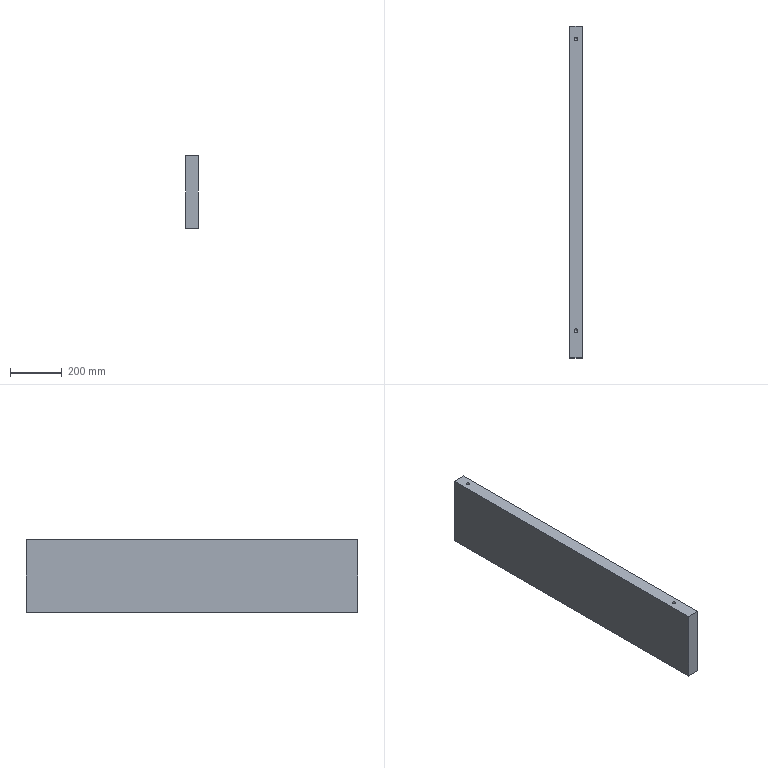Part | NX | features 29 2 | 1 solid | 16 faces | box 50 x 1280 x 280.5 mm | volume 17921318 mm3 | plane 6 | cylinder 5 | cone 5 | commonest cylinder face diameters 14.1 x5
STEP:
#1=CARTESIAN_POINT('',(2407.05,622.5,-493.5));
#2=VERTEX_POINT('',#1);
#3=CARTESIAN_POINT('',(2400.,622.5,-493.5));
#4=DIRECTION('',(0.,0.,1.));
#5=DIRECTION('',(1.,0.,0.));
#6=AXIS2_PLACEMENT_3D('',#3,#4,#5);
#7=CIRCLE('',#6,7.05);
#8=EDGE_CURVE('',#2,#2,#7,.T.);
#9=ORIENTED_EDGE('',*,*,#8,.T.);
#10=EDGE_LOOP('',(#9));
#11=FACE_BOUND('',#10,.T.);
#12=CARTESIAN_POINT('',(2375.,-607.5,-493.5));
#13=VERTEX_POINT('',#12);
#14=CARTESIAN_POINT('',(2425.,-607.5,-493.5));
#15=VERTEX_POINT('',#14);
#16=CARTESIAN_POINT('',(2330.,-607.5,-493.5));
#17=DIRECTION('',(1.,0.,0.));
#18=VECTOR('',#17,1000.);
#19=LINE('',#16,#18);
#20=EDGE_CURVE('',#13,#15,#19,.T.);
#21=ORIENTED_EDGE('',*,*,#20,.F.);
#22=CARTESIAN_POINT('',(2375.,672.5,-493.5));
#23=VERTEX_POINT('',#22);
#24=CARTESIAN_POINT('',(2375.,193.,-493.5));
#25=DIRECTION('',(0.,-1.,0.));
#26=VECTOR('',#25,1000.);
#27=LINE('',#24,#26);
#28=EDGE_CURVE('',#23,#13,#27,.T.);
#29=ORIENTED_EDGE('',*,*,#28,.F.);
#30=CARTESIAN_POINT('',(2425.,672.5,-493.5));
#31=VERTEX_POINT('',#30);
#32=CARTESIAN_POINT('',(1932.5,672.5,-493.5));
#33=DIRECTION('',(1.,0.,0.));
#34=VECTOR('',#33,1000.);
#35=LINE('',#32,#34);
#36=EDGE_CURVE('',#23,#31,#35,.T.);
#37=ORIENTED_EDGE('',*,*,#36,.T.);
#38=CARTESIAN_POINT('',(2425.,193.,-493.5));
#39=DIRECTION('',(0.,1.,0.));
#40=VECTOR('',#39,1000.);
#41=LINE('',#38,#40);
#42=EDGE_CURVE('',#15,#31,#41,.T.);
#43=ORIENTED_EDGE('',*,*,#42,.F.);
#44=EDGE_LOOP('',(#21,#29,#37,#43));
#45=FACE_BOUND('',#44,.T.);
#46=CARTESIAN_POINT('',(2407.05,-502.5,-493.5));
#47=VERTEX_POINT('',#46);
#48=CARTESIAN_POINT('',(2400.,-502.5,-493.5));
#49=DIRECTION('',(0.,0.,1.));
#50=DIRECTION('',(1.,0.,0.));
#51=AXIS2_PLACEMENT_3D('',#48,#49,#50);
#52=CIRCLE('',#51,7.05);
#53=EDGE_CURVE('',#47,#47,#52,.T.);
#54=ORIENTED_EDGE('',*,*,#53,.T.);
#55=EDGE_LOOP('',(#54));
#56=FACE_BOUND('',#55,.T.);
#57=CARTESIAN_POINT('',(2407.05,32.5,-493.5));
#58=VERTEX_POINT('',#57);
#59=CARTESIAN_POINT('',(2400.,32.5,-493.5));
#60=DIRECTION('',(0.,0.,1.));
#61=DIRECTION('',(1.,0.,0.));
#62=AXIS2_PLACEMENT_3D('',#59,#60,#61);
#63=CIRCLE('',#62,7.05);
#64=EDGE_CURVE('',#58,#58,#63,.T.);
#65=ORIENTED_EDGE('',*,*,#64,.T.);
#66=EDGE_LOOP('',(#65));
#67=FACE_BOUND('',#66,.T.);
#68=CARTESIAN_POINT('',(1945.,0.,-493.5));
#69=DIRECTION('',(0.,0.,-1.));
#70=DIRECTION('',(1.,0.,0.));
#71=AXIS2_PLACEMENT_3D('',#68,#69,#70);
#72=PLANE('',#71);
#73=ADVANCED_FACE('',(#11,#45,#56,#67),#72,.T.);
#74=CARTESIAN_POINT('',(2407.05,622.5,-213.));
#75=VERTEX_POINT('',#74);
#76=CARTESIAN_POINT('',(2400.,622.5,-213.));
#77=DIRECTION('',(0.,0.,-1.));
#78=DIRECTION('',(1.,0.,0.));
#79=AXIS2_PLACEMENT_3D('',#76,#77,#78);
#80=CIRCLE('',#79,7.05);
#81=EDGE_CURVE('',#75,#75,#80,.T.);
#82=ORIENTED_EDGE('',*,*,#81,.T.);
#83=EDGE_LOOP('',(#82));
#84=FACE_BOUND('',#83,.T.);
#85=CARTESIAN_POINT('',(2425.,-607.5,-213.));
#86=VERTEX_POINT('',#85);
#87=CARTESIAN_POINT('',(2375.,-607.5,-213.));
#88=VERTEX_POINT('',#87);
#89=CARTESIAN_POINT('',(2330.,-607.5,-213.));
#90=DIRECTION('',(-1.,0.,0.));
#91=VECTOR('',#90,1000.);
#92=LINE('',#89,#91);
#93=EDGE_CURVE('',#86,#88,#92,.T.);
#94=ORIENTED_EDGE('',*,*,#93,.F.);
#95=CARTESIAN_POINT('',(2425.,672.5,-213.));
#96=VERTEX_POINT('',#95);
#97=CARTESIAN_POINT('',(2425.,193.,-213.));
#98=DIRECTION('',(0.,-1.,0.));
#99=VECTOR('',#98,1000.);
#100=LINE('',#97,#99);
#101=EDGE_CURVE('',#96,#86,#100,.T.);
#102=ORIENTED_EDGE('',*,*,#101,.F.);
#103=CARTESIAN_POINT('',(2375.,672.5,-213.));
#104=VERTEX_POINT('',#103);
#105=CARTESIAN_POINT('',(1932.5,672.5,-213.));
#106=DIRECTION('',(-1.,0.,0.));
#107=VECTOR('',#106,1000.);
#108=LINE('',#105,#107);
#109=EDGE_CURVE('',#96,#104,#108,.T.);
#110=ORIENTED_EDGE('',*,*,#109,.T.);
#111=CARTESIAN_POINT('',(2375.,193.,-213.));
#112=DIRECTION('',(0.,1.,0.));
#113=VECTOR('',#112,1000.);
#114=LINE('',#111,#113);
#115=EDGE_CURVE('',#88,#104,#114,.T.);
#116=ORIENTED_EDGE('',*,*,#115,.F.);
#117=EDGE_LOOP('',(#94,#102,#110,#116));
#118=FACE_BOUND('',#117,.T.);
#119=CARTESIAN_POINT('',(2407.05,-502.5,-213.));
#120=VERTEX_POINT('',#119);
#121=CARTESIAN_POINT('',(2400.,-502.5,-213.));
#122=DIRECTION('',(0.,0.,-1.));
#123=DIRECTION('',(1.,0.,0.));
#124=AXIS2_PLACEMENT_3D('',#121,#122,#123);
#125=CIRCLE('',#124,7.05);
#126=EDGE_CURVE('',#120,#120,#125,.T.);
#127=ORIENTED_EDGE('',*,*,#126,.T.);
#128=EDGE_LOOP('',(#127));
#129=FACE_BOUND('',#128,.T.);
#130=CARTESIAN_POINT('',(1945.,0.,-213.));
#131=DIRECTION('',(0.,0.,1.));
#132=DIRECTION('',(-1.,0.,0.));
#133=AXIS2_PLACEMENT_3D('',#130,#131,#132);
#134=PLANE('',#133);
#135=ADVANCED_FACE('',(#84,#118,#129),#134,.T.);
#136=CARTESIAN_POINT('',(2375.,-607.5,-205.5));
#137=DIRECTION('',(0.,0.,1.));
#138=VECTOR('',#137,1000.);
#139=LINE('',#136,#138);
#140=EDGE_CURVE('',#13,#88,#139,.T.);
#141=ORIENTED_EDGE('',*,*,#140,.F.);
#142=ORIENTED_EDGE('',*,*,#20,.T.);
#143=CARTESIAN_POINT('',(2425.,-607.5,-205.5));
#144=DIRECTION('',(0.,0.,-1.));
#145=VECTOR('',#144,1000.);
#146=LINE('',#143,#145);
#147=EDGE_CURVE('',#86,#15,#146,.T.);
#148=ORIENTED_EDGE('',*,*,#147,.F.);
#149=ORIENTED_EDGE('',*,*,#93,.T.);
#150=EDGE_LOOP('',(#141,#142,#148,#149));
#151=FACE_BOUND('',#150,.T.);
#152=CARTESIAN_POINT('',(2330.,-607.5,-446.));
#153=DIRECTION('',(0.,-1.,0.));
#154=DIRECTION('',(0.,0.,1.));
#155=AXIS2_PLACEMENT_3D('',#152,#153,#154);
#156=PLANE('',#155);
#157=ADVANCED_FACE('',(#151),#156,.T.);
#158=CARTESIAN_POINT('',(2375.,672.5,-205.5));
#159=DIRECTION('',(0.,0.,1.));
#160=VECTOR('',#159,1000.);
#161=LINE('',#158,#160);
#162=EDGE_CURVE('',#23,#104,#161,.T.);
#163=ORIENTED_EDGE('',*,*,#162,.F.);
#164=ORIENTED_EDGE('',*,*,#28,.T.);
#165=ORIENTED_EDGE('',*,*,#140,.T.);
#166=ORIENTED_EDGE('',*,*,#115,.T.);
#167=EDGE_LOOP('',(#163,#164,#165,#166));
#168=FACE_BOUND('',#167,.T.);
#169=CARTESIAN_POINT('',(2375.,193.,-205.5));
#170=DIRECTION('',(-1.,0.,0.));
#171=DIRECTION('',(0.,0.,1.));
#172=AXIS2_PLACEMENT_3D('',#169,#170,#171);
#173=PLANE('',#172);
#174=ADVANCED_FACE('',(#168),#173,.T.);
#175=ORIENTED_EDGE('',*,*,#147,.T.);
#176=ORIENTED_EDGE('',*,*,#42,.T.);
#177=CARTESIAN_POINT('',(2425.,672.5,91.));
#178=DIRECTION('',(0.,0.,1.));
#179=VECTOR('',#178,1000.);
#180=LINE('',#177,#179);
#181=EDGE_CURVE('',#31,#96,#180,.T.);
#182=ORIENTED_EDGE('',*,*,#181,.T.);
#183=ORIENTED_EDGE('',*,*,#101,.T.);
#184=EDGE_LOOP('',(#175,#176,#182,#183));
#185=FACE_BOUND('',#184,.T.);
#186=CARTESIAN_POINT('',(2425.,193.,-205.5));
#187=DIRECTION('',(1.,0.,0.));
#188=DIRECTION('',(0.,0.,-1.));
#189=AXIS2_PLACEMENT_3D('',#186,#187,#188);
#190=PLANE('',#189);
#191=ADVANCED_FACE('',(#185),#190,.T.);
#192=ORIENTED_EDGE('',*,*,#36,.F.);
#193=ORIENTED_EDGE('',*,*,#162,.T.);
#194=ORIENTED_EDGE('',*,*,#109,.F.);
#195=ORIENTED_EDGE('',*,*,#181,.F.);
#196=EDGE_LOOP('',(#192,#193,#194,#195));
#197=FACE_BOUND('',#196,.T.);
#198=CARTESIAN_POINT('',(1932.5,672.5,91.));
#199=DIRECTION('',(0.,-1.,0.));
#200=DIRECTION('',(-1.,0.,0.));
#201=AXIS2_PLACEMENT_3D('',#198,#199,#200);
#202=PLANE('',#201);
#203=ADVANCED_FACE('',(#197),#202,.F.);
#204=CARTESIAN_POINT('',(2392.95,622.5,-249.95));
#205=VERTEX_POINT('',#204);
#206=CARTESIAN_POINT('',(2400.,622.5,-249.95));
#207=DIRECTION('',(0.,0.,-1.));
#208=DIRECTION('',(-1.,0.,0.));
#209=AXIS2_PLACEMENT_3D('',#206,#207,#208);
#210=CIRCLE('',#209,7.05);
#211=EDGE_CURVE('',#205,#205,#210,.T.);
#212=ORIENTED_EDGE('',*,*,#211,.T.);
#213=EDGE_LOOP('',(#212));
#214=FACE_BOUND('',#213,.T.);
#215=ORIENTED_EDGE('',*,*,#81,.F.);
#216=EDGE_LOOP('',(#215));
#217=FACE_BOUND('',#216,.T.);
#218=CARTESIAN_POINT('',(2400.,622.5,-213.));
#219=DIRECTION('',(0.,0.,-1.));
#220=DIRECTION('',(-1.,0.,0.));
#221=AXIS2_PLACEMENT_3D('',#218,#219,#220);
#222=CYLINDRICAL_SURFACE('',#221,7.05);
#223=ADVANCED_FACE('',(#214,#217),#222,.F.);
#224=CARTESIAN_POINT('',(2400.,622.5,-257.));
#225=VERTEX_POINT('',#224);
#226=VERTEX_LOOP('',#225);
#227=FACE_BOUND('',#226,.T.);
#228=ORIENTED_EDGE('',*,*,#211,.F.);
#229=EDGE_LOOP('',(#228));
#230=FACE_BOUND('',#229,.T.);
#231=CARTESIAN_POINT('',(2400.,622.5,-249.95));
#232=DIRECTION('',(0.,0.,1.));
#233=DIRECTION('',(-1.,0.,0.));
#234=AXIS2_PLACEMENT_3D('',#231,#232,#233);
#235=CONICAL_SURFACE('',#234,7.05,0.7854);
#236=ADVANCED_FACE('',(#227,#230),#235,.F.);
#237=CARTESIAN_POINT('',(2392.95,-502.5,-249.95));
#238=VERTEX_POINT('',#237);
#239=CARTESIAN_POINT('',(2400.,-502.5,-249.95));
#240=DIRECTION('',(0.,0.,-1.));
#241=DIRECTION('',(-1.,0.,0.));
#242=AXIS2_PLACEMENT_3D('',#239,#240,#241);
#243=CIRCLE('',#242,7.05);
#244=EDGE_CURVE('',#238,#238,#243,.T.);
#245=ORIENTED_EDGE('',*,*,#244,.T.);
#246=EDGE_LOOP('',(#245));
#247=FACE_BOUND('',#246,.T.);
#248=ORIENTED_EDGE('',*,*,#126,.F.);
#249=EDGE_LOOP('',(#248));
#250=FACE_BOUND('',#249,.T.);
#251=CARTESIAN_POINT('',(2400.,-502.5,-213.));
#252=DIRECTION('',(0.,0.,-1.));
#253=DIRECTION('',(-1.,0.,0.));
#254=AXIS2_PLACEMENT_3D('',#251,#252,#253);
#255=CYLINDRICAL_SURFACE('',#254,7.05);
#256=ADVANCED_FACE('',(#247,#250),#255,.F.);
#257=CARTESIAN_POINT('',(2400.,-502.5,-257.));
#258=VERTEX_POINT('',#257);
#259=VERTEX_LOOP('',#258);
#260=FACE_BOUND('',#259,.T.);
#261=ORIENTED_EDGE('',*,*,#244,.F.);
#262=EDGE_LOOP('',(#261));
#263=FACE_BOUND('',#262,.T.);
#264=CARTESIAN_POINT('',(2400.,-502.5,-249.95));
#265=DIRECTION('',(0.,0.,1.));
#266=DIRECTION('',(-1.,0.,0.));
#267=AXIS2_PLACEMENT_3D('',#264,#265,#266);
#268=CONICAL_SURFACE('',#267,7.05,0.7854);
#269=ADVANCED_FACE('',(#260,#263),#268,.F.);
#270=CARTESIAN_POINT('',(2407.05,-502.5,-456.55));
#271=VERTEX_POINT('',#270);
#272=CARTESIAN_POINT('',(2400.,-502.5,-456.55));
#273=DIRECTION('',(0.,0.,1.));
#274=DIRECTION('',(1.,0.,0.));
#275=AXIS2_PLACEMENT_3D('',#272,#273,#274);
#276=CIRCLE('',#275,7.05);
#277=EDGE_CURVE('',#271,#271,#276,.T.);
#278=ORIENTED_EDGE('',*,*,#277,.T.);
#279=EDGE_LOOP('',(#278));
#280=FACE_BOUND('',#279,.T.);
#281=ORIENTED_EDGE('',*,*,#53,.F.);
#282=EDGE_LOOP('',(#281));
#283=FACE_BOUND('',#282,.T.);
#284=CARTESIAN_POINT('',(2400.,-502.5,-493.5));
#285=DIRECTION('',(0.,0.,1.));
#286=DIRECTION('',(-1.,0.,0.));
#287=AXIS2_PLACEMENT_3D('',#284,#285,#286);
#288=CYLINDRICAL_SURFACE('',#287,7.05);
#289=ADVANCED_FACE('',(#280,#283),#288,.F.);
#290=CARTESIAN_POINT('',(2400.,-502.5,-449.5));
#291=VERTEX_POINT('',#290);
#292=VERTEX_LOOP('',#291);
#293=FACE_BOUND('',#292,.T.);
#294=ORIENTED_EDGE('',*,*,#277,.F.);
#295=EDGE_LOOP('',(#294));
#296=FACE_BOUND('',#295,.T.);
#297=CARTESIAN_POINT('',(2400.,-502.5,-456.55));
#298=DIRECTION('',(0.,0.,-1.));
#299=DIRECTION('',(1.,0.,0.));
#300=AXIS2_PLACEMENT_3D('',#297,#298,#299);
#301=CONICAL_SURFACE('',#300,7.05,0.7854);
#302=ADVANCED_FACE('',(#293,#296),#301,.F.);
#303=CARTESIAN_POINT('',(2407.05,622.5,-456.55));
#304=VERTEX_POINT('',#303);
#305=CARTESIAN_POINT('',(2400.,622.5,-456.55));
#306=DIRECTION('',(0.,0.,1.));
#307=DIRECTION('',(1.,0.,0.));
#308=AXIS2_PLACEMENT_3D('',#305,#306,#307);
#309=CIRCLE('',#308,7.05);
#310=EDGE_CURVE('',#304,#304,#309,.T.);
#311=ORIENTED_EDGE('',*,*,#310,.T.);
#312=EDGE_LOOP('',(#311));
#313=FACE_BOUND('',#312,.T.);
#314=ORIENTED_EDGE('',*,*,#8,.F.);
#315=EDGE_LOOP('',(#314));
#316=FACE_BOUND('',#315,.T.);
#317=CARTESIAN_POINT('',(2400.,622.5,-493.5));
#318=DIRECTION('',(0.,0.,1.));
#319=DIRECTION('',(-1.,0.,0.));
#320=AXIS2_PLACEMENT_3D('',#317,#318,#319);
#321=CYLINDRICAL_SURFACE('',#320,7.05);
#322=ADVANCED_FACE('',(#313,#316),#321,.F.);
#323=CARTESIAN_POINT('',(2400.,622.5,-449.5));
#324=VERTEX_POINT('',#323);
#325=VERTEX_LOOP('',#324);
#326=FACE_BOUND('',#325,.T.);
#327=ORIENTED_EDGE('',*,*,#310,.F.);
#328=EDGE_LOOP('',(#327));
#329=FACE_BOUND('',#328,.T.);
#330=CARTESIAN_POINT('',(2400.,622.5,-456.55));
#331=DIRECTION('',(0.,0.,-1.));
#332=DIRECTION('',(1.,0.,0.));
#333=AXIS2_PLACEMENT_3D('',#330,#331,#332);
#334=CONICAL_SURFACE('',#333,7.05,0.7854);
#335=ADVANCED_FACE('',(#326,#329),#334,.F.);
#336=CARTESIAN_POINT('',(2407.05,32.5,-456.55));
#337=VERTEX_POINT('',#336);
#338=CARTESIAN_POINT('',(2400.,32.5,-456.55));
#339=DIRECTION('',(0.,0.,1.));
#340=DIRECTION('',(1.,0.,0.));
#341=AXIS2_PLACEMENT_3D('',#338,#339,#340);
#342=CIRCLE('',#341,7.05);
#343=EDGE_CURVE('',#337,#337,#342,.T.);
#344=ORIENTED_EDGE('',*,*,#343,.T.);
#345=EDGE_LOOP('',(#344));
#346=FACE_BOUND('',#345,.T.);
#347=ORIENTED_EDGE('',*,*,#64,.F.);
#348=EDGE_LOOP('',(#347));
#349=FACE_BOUND('',#348,.T.);
#350=CARTESIAN_POINT('',(2400.,32.5,-493.5));
#351=DIRECTION('',(0.,0.,1.));
#352=DIRECTION('',(-1.,0.,0.));
#353=AXIS2_PLACEMENT_3D('',#350,#351,#352);
#354=CYLINDRICAL_SURFACE('',#353,7.05);
#355=ADVANCED_FACE('',(#346,#349),#354,.F.);
#356=CARTESIAN_POINT('',(2400.,32.5,-449.5));
#357=VERTEX_POINT('',#356);
#358=VERTEX_LOOP('',#357);
#359=FACE_BOUND('',#358,.T.);
#360=ORIENTED_EDGE('',*,*,#343,.F.);
#361=EDGE_LOOP('',(#360));
#362=FACE_BOUND('',#361,.T.);
#363=CARTESIAN_POINT('',(2400.,32.5,-456.55));
#364=DIRECTION('',(0.,0.,-1.));
#365=DIRECTION('',(1.,0.,0.));
#366=AXIS2_PLACEMENT_3D('',#363,#364,#365);
#367=CONICAL_SURFACE('',#366,7.05,0.7854);
#368=ADVANCED_FACE('',(#359,#362),#367,.F.);
#369=CLOSED_SHELL('',(#73,#135,#157,#174,#191,#203,#223,#236,#256,#269,#289,#302,#322,#335,#355,#368));
#370=MANIFOLD_SOLID_BREP('',#369);
#371=(LENGTH_UNIT()NAMED_UNIT(*)SI_UNIT(.MILLI.,.METRE.));
#372=UNCERTAINTY_MEASURE_WITH_UNIT(LENGTH_MEASURE(0.00001),#371,'','');
#373=(NAMED_UNIT(*)PLANE_ANGLE_UNIT()SI_UNIT($,.RADIAN.));
#374=(NAMED_UNIT(*)SI_UNIT($,.STERADIAN.)SOLID_ANGLE_UNIT());
#375=(GEOMETRIC_REPRESENTATION_CONTEXT(3)GLOBAL_UNCERTAINTY_ASSIGNED_CONTEXT((#372))GLOBAL_UNIT_ASSIGNED_CONTEXT((#371,#373,#374))REPRESENTATION_CONTEXT('',''));
#376=ADVANCED_BREP_SHAPE_REPRESENTATION('',(#370),#375);